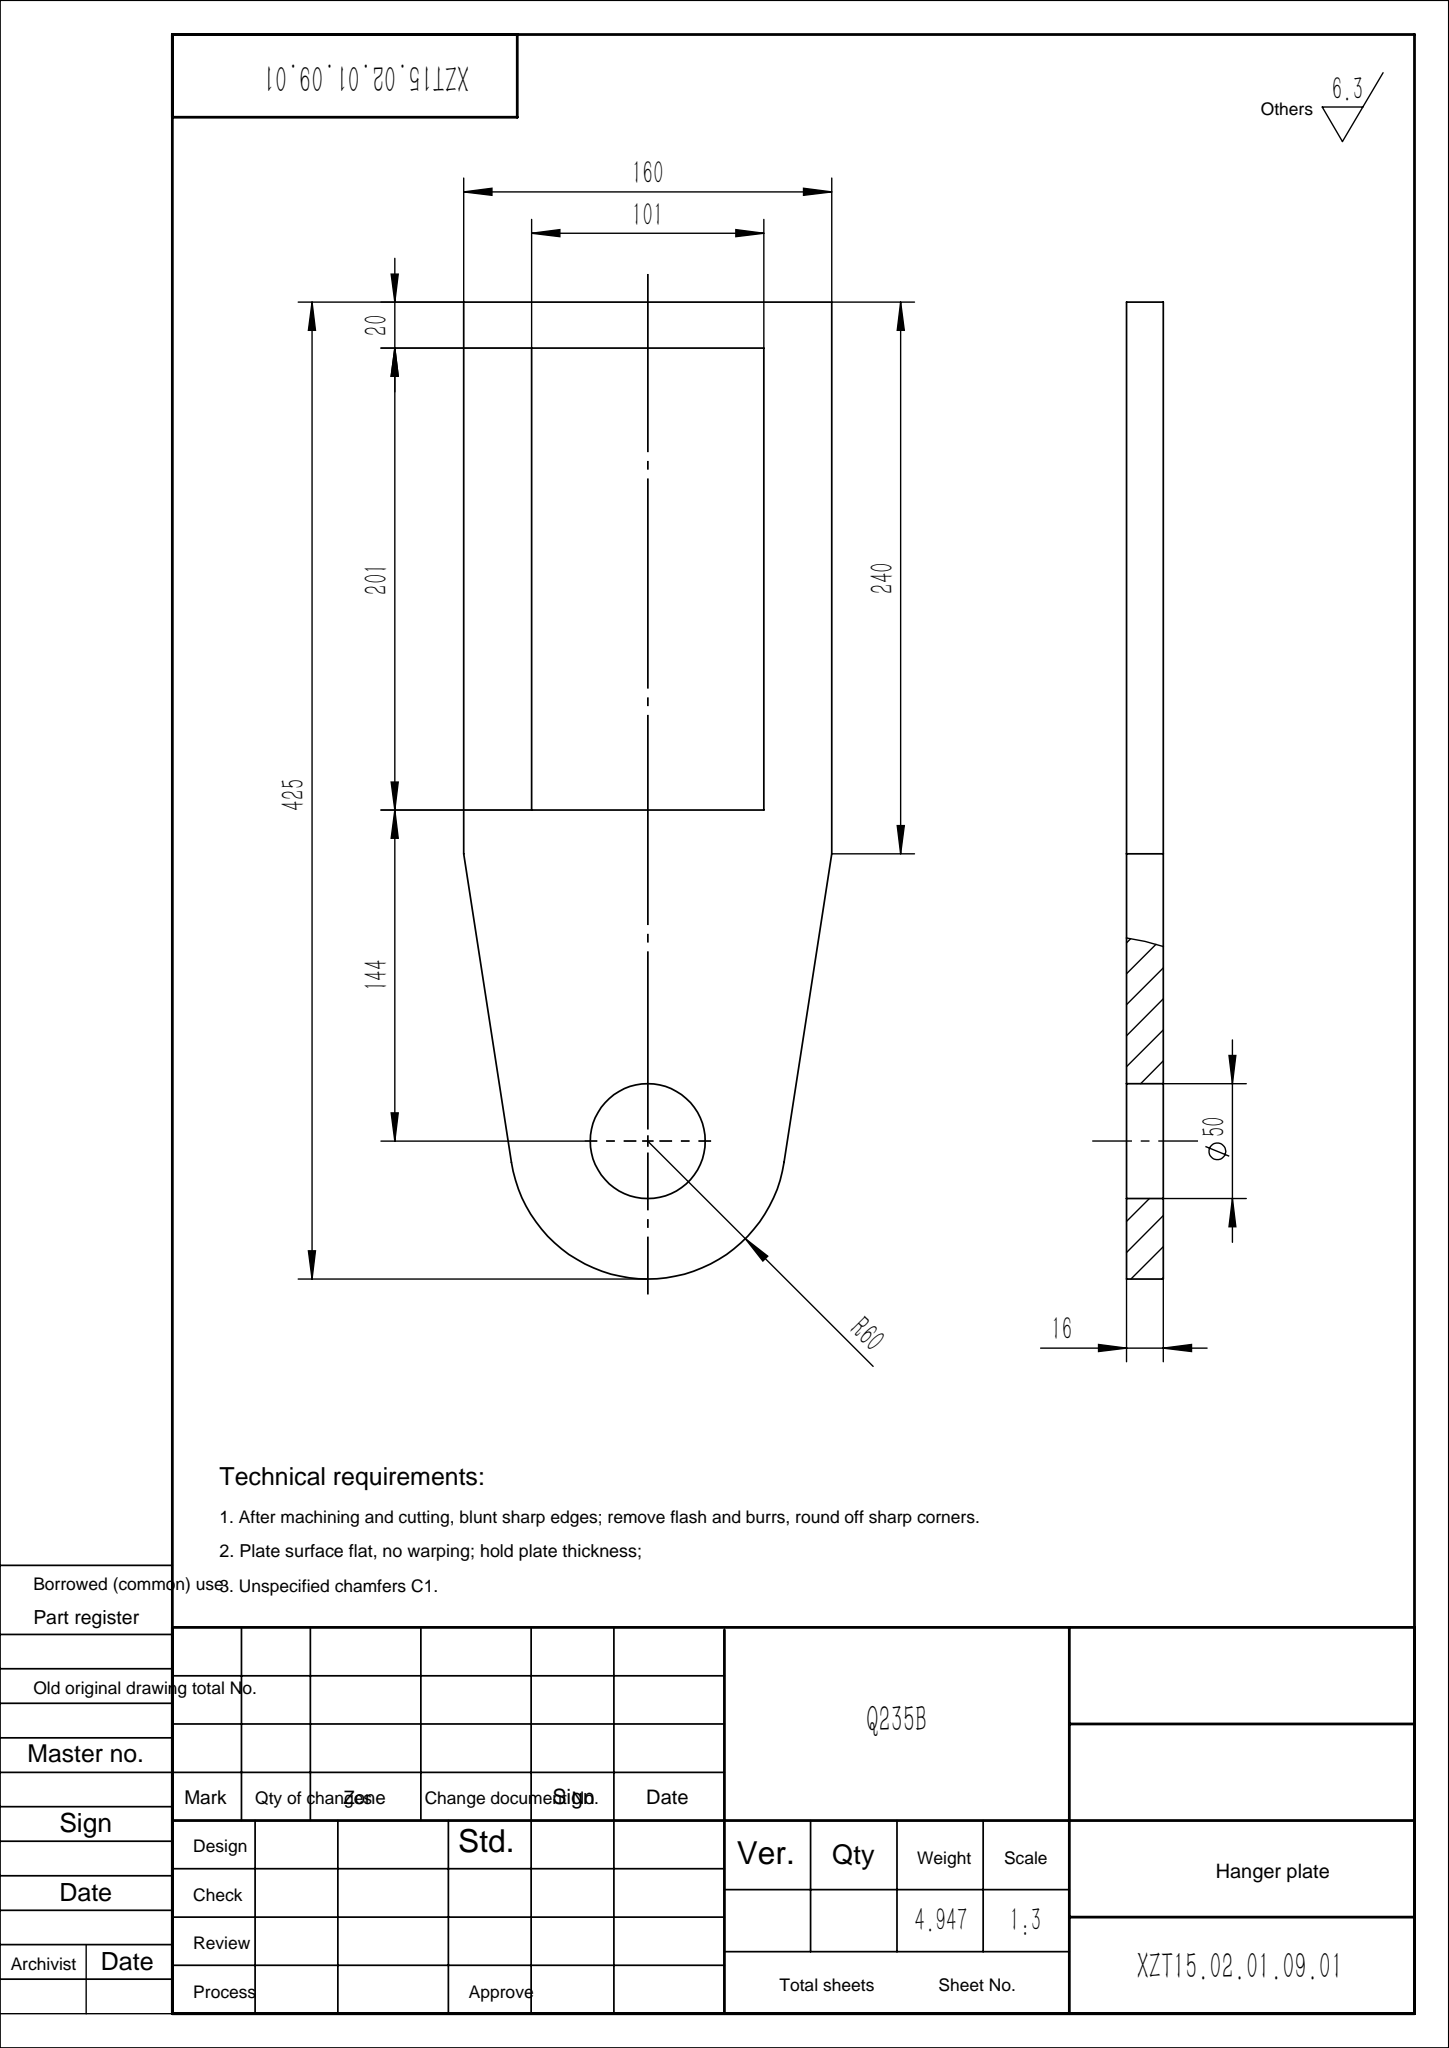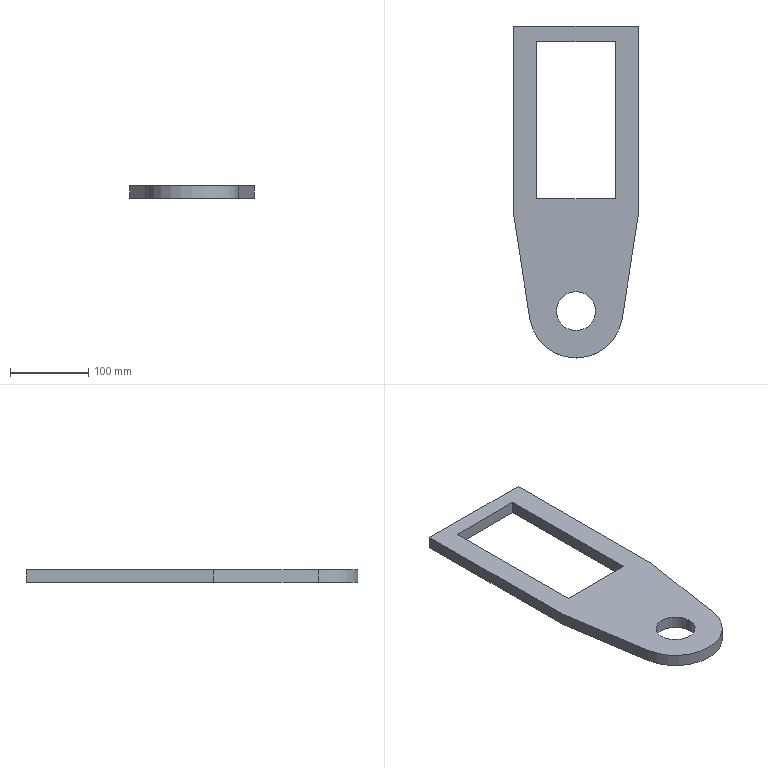Part | SolidWorks | features Extrusion 1 | 1 solid | 14 faces | box 160 x 425 x 16 mm | volume 630136 mm3 | plane 11 | cylinder 3 | commonest cylinder face diameters 50 x2 120 x1
STEP:
#1=CARTESIAN_POINT('',(-25.,0.,8.));
#2=VERTEX_POINT('',#1);
#3=CARTESIAN_POINT('',(25.,0.,8.));
#4=VERTEX_POINT('',#3);
#5=CARTESIAN_POINT('',(0.,0.,8.));
#6=DIRECTION('',(0.,0.,1.));
#7=DIRECTION('',(1.,0.,0.));
#8=AXIS2_PLACEMENT_3D('',#5,#6,#7);
#9=CIRCLE('',#8,25.);
#10=EDGE_CURVE('',#2,#4,#9,.T.);
#11=ORIENTED_EDGE('',*,*,#10,.T.);
#12=CARTESIAN_POINT('',(25.,0.,-8.));
#13=VERTEX_POINT('',#12);
#14=CARTESIAN_POINT('',(25.,0.,8.));
#15=DIRECTION('',(0.,0.,-1.));
#16=VECTOR('',#15,1000.);
#17=LINE('',#14,#16);
#18=EDGE_CURVE('',#4,#13,#17,.T.);
#19=ORIENTED_EDGE('',*,*,#18,.T.);
#20=CARTESIAN_POINT('',(-25.,0.,-8.));
#21=VERTEX_POINT('',#20);
#22=CARTESIAN_POINT('',(0.,0.,-8.));
#23=DIRECTION('',(0.,0.,1.));
#24=DIRECTION('',(1.,0.,0.));
#25=AXIS2_PLACEMENT_3D('',#22,#23,#24);
#26=CIRCLE('',#25,25.);
#27=EDGE_CURVE('',#21,#13,#26,.T.);
#28=ORIENTED_EDGE('',*,*,#27,.F.);
#29=CARTESIAN_POINT('',(-25.,0.,8.));
#30=DIRECTION('',(0.,0.,-1.));
#31=VECTOR('',#30,1000.);
#32=LINE('',#29,#31);
#33=EDGE_CURVE('',#2,#21,#32,.T.);
#34=ORIENTED_EDGE('',*,*,#33,.F.);
#35=EDGE_LOOP('',(#11,#19,#28,#34));
#36=FACE_OUTER_BOUND('',#35,.T.);
#37=CARTESIAN_POINT('',(0.,0.,8.));
#38=DIRECTION('',(0.,0.,-1.));
#39=DIRECTION('',(-1.,0.,0.));
#40=AXIS2_PLACEMENT_3D('',#37,#38,#39);
#41=CYLINDRICAL_SURFACE('',#40,25.);
#42=ADVANCED_FACE('',(#36),#41,.F.);
#43=CARTESIAN_POINT('',(-80.,365.,8.));
#44=VERTEX_POINT('',#43);
#45=CARTESIAN_POINT('',(-80.,125.,8.));
#46=VERTEX_POINT('',#45);
#47=CARTESIAN_POINT('',(-80.,365.,8.));
#48=DIRECTION('',(0.,-1.,0.));
#49=VECTOR('',#48,1000.);
#50=LINE('',#47,#49);
#51=EDGE_CURVE('',#44,#46,#50,.T.);
#52=ORIENTED_EDGE('',*,*,#51,.T.);
#53=CARTESIAN_POINT('',(-59.298,-9.151,8.));
#54=VERTEX_POINT('',#53);
#55=CARTESIAN_POINT('',(-80.,125.,8.));
#56=DIRECTION('',(0.1525,-0.9883,0.));
#57=VECTOR('',#56,1000.);
#58=LINE('',#55,#57);
#59=EDGE_CURVE('',#46,#54,#58,.T.);
#60=ORIENTED_EDGE('',*,*,#59,.T.);
#61=CARTESIAN_POINT('',(59.298,-9.151,8.));
#62=VERTEX_POINT('',#61);
#63=CARTESIAN_POINT('',(0.,0.,8.));
#64=DIRECTION('',(0.,0.,1.));
#65=DIRECTION('',(1.,0.,0.));
#66=AXIS2_PLACEMENT_3D('',#63,#64,#65);
#67=CIRCLE('',#66,60.);
#68=EDGE_CURVE('',#54,#62,#67,.T.);
#69=ORIENTED_EDGE('',*,*,#68,.T.);
#70=CARTESIAN_POINT('',(80.,125.,8.));
#71=VERTEX_POINT('',#70);
#72=CARTESIAN_POINT('',(80.,125.,8.));
#73=DIRECTION('',(0.1525,0.9883,0.));
#74=VECTOR('',#73,1000.);
#75=LINE('',#72,#74);
#76=EDGE_CURVE('',#62,#71,#75,.T.);
#77=ORIENTED_EDGE('',*,*,#76,.T.);
#78=CARTESIAN_POINT('',(80.,365.,8.));
#79=VERTEX_POINT('',#78);
#80=CARTESIAN_POINT('',(80.,365.,8.));
#81=DIRECTION('',(0.,1.,0.));
#82=VECTOR('',#81,1000.);
#83=LINE('',#80,#82);
#84=EDGE_CURVE('',#71,#79,#83,.T.);
#85=ORIENTED_EDGE('',*,*,#84,.T.);
#86=CARTESIAN_POINT('',(80.,365.,8.));
#87=DIRECTION('',(-1.,0.,0.));
#88=VECTOR('',#87,1000.);
#89=LINE('',#86,#88);
#90=EDGE_CURVE('',#79,#44,#89,.T.);
#91=ORIENTED_EDGE('',*,*,#90,.T.);
#92=EDGE_LOOP('',(#52,#60,#69,#77,#85,#91));
#93=FACE_OUTER_BOUND('',#92,.T.);
#94=ORIENTED_EDGE('',*,*,#10,.F.);
#95=CARTESIAN_POINT('',(0.,0.,8.));
#96=DIRECTION('',(0.,0.,1.));
#97=DIRECTION('',(1.,0.,0.));
#98=AXIS2_PLACEMENT_3D('',#95,#96,#97);
#99=CIRCLE('',#98,25.);
#100=EDGE_CURVE('',#4,#2,#99,.T.);
#101=ORIENTED_EDGE('',*,*,#100,.F.);
#102=EDGE_LOOP('',(#94,#101));
#103=FACE_BOUND('',#102,.T.);
#104=CARTESIAN_POINT('',(-50.5,144.,8.));
#105=VERTEX_POINT('',#104);
#106=CARTESIAN_POINT('',(50.5,144.,8.));
#107=VERTEX_POINT('',#106);
#108=CARTESIAN_POINT('',(50.5,144.,8.));
#109=DIRECTION('',(1.,0.,0.));
#110=VECTOR('',#109,1000.);
#111=LINE('',#108,#110);
#112=EDGE_CURVE('',#105,#107,#111,.T.);
#113=ORIENTED_EDGE('',*,*,#112,.F.);
#114=CARTESIAN_POINT('',(-50.5,345.,8.));
#115=VERTEX_POINT('',#114);
#116=CARTESIAN_POINT('',(-50.5,144.,8.));
#117=DIRECTION('',(0.,-1.,0.));
#118=VECTOR('',#117,1000.);
#119=LINE('',#116,#118);
#120=EDGE_CURVE('',#115,#105,#119,.T.);
#121=ORIENTED_EDGE('',*,*,#120,.F.);
#122=CARTESIAN_POINT('',(50.5,345.,8.));
#123=VERTEX_POINT('',#122);
#124=CARTESIAN_POINT('',(50.5,345.,8.));
#125=DIRECTION('',(-1.,0.,0.));
#126=VECTOR('',#125,1000.);
#127=LINE('',#124,#126);
#128=EDGE_CURVE('',#123,#115,#127,.T.);
#129=ORIENTED_EDGE('',*,*,#128,.F.);
#130=CARTESIAN_POINT('',(50.5,144.,8.));
#131=DIRECTION('',(0.,1.,0.));
#132=VECTOR('',#131,1000.);
#133=LINE('',#130,#132);
#134=EDGE_CURVE('',#107,#123,#133,.T.);
#135=ORIENTED_EDGE('',*,*,#134,.F.);
#136=EDGE_LOOP('',(#113,#121,#129,#135));
#137=FACE_BOUND('',#136,.T.);
#138=CARTESIAN_POINT('',(0.,0.,8.));
#139=DIRECTION('',(0.,0.,1.));
#140=DIRECTION('',(1.,0.,0.));
#141=AXIS2_PLACEMENT_3D('',#138,#139,#140);
#142=PLANE('',#141);
#143=ADVANCED_FACE('',(#93,#103,#137),#142,.T.);
#144=ORIENTED_EDGE('',*,*,#27,.T.);
#145=CARTESIAN_POINT('',(0.,0.,-8.));
#146=DIRECTION('',(0.,0.,1.));
#147=DIRECTION('',(1.,0.,0.));
#148=AXIS2_PLACEMENT_3D('',#145,#146,#147);
#149=CIRCLE('',#148,25.);
#150=EDGE_CURVE('',#13,#21,#149,.T.);
#151=ORIENTED_EDGE('',*,*,#150,.T.);
#152=EDGE_LOOP('',(#144,#151));
#153=FACE_BOUND('',#152,.T.);
#154=CARTESIAN_POINT('',(-80.,365.,-8.));
#155=VERTEX_POINT('',#154);
#156=CARTESIAN_POINT('',(-80.,125.,-8.));
#157=VERTEX_POINT('',#156);
#158=CARTESIAN_POINT('',(-80.,365.,-8.));
#159=DIRECTION('',(0.,-1.,0.));
#160=VECTOR('',#159,1000.);
#161=LINE('',#158,#160);
#162=EDGE_CURVE('',#155,#157,#161,.T.);
#163=ORIENTED_EDGE('',*,*,#162,.F.);
#164=CARTESIAN_POINT('',(80.,365.,-8.));
#165=VERTEX_POINT('',#164);
#166=CARTESIAN_POINT('',(80.,365.,-8.));
#167=DIRECTION('',(-1.,0.,0.));
#168=VECTOR('',#167,1000.);
#169=LINE('',#166,#168);
#170=EDGE_CURVE('',#165,#155,#169,.T.);
#171=ORIENTED_EDGE('',*,*,#170,.F.);
#172=CARTESIAN_POINT('',(80.,125.,-8.));
#173=VERTEX_POINT('',#172);
#174=CARTESIAN_POINT('',(80.,365.,-8.));
#175=DIRECTION('',(0.,1.,0.));
#176=VECTOR('',#175,1000.);
#177=LINE('',#174,#176);
#178=EDGE_CURVE('',#173,#165,#177,.T.);
#179=ORIENTED_EDGE('',*,*,#178,.F.);
#180=CARTESIAN_POINT('',(59.298,-9.151,-8.));
#181=VERTEX_POINT('',#180);
#182=CARTESIAN_POINT('',(80.,125.,-8.));
#183=DIRECTION('',(0.1525,0.9883,0.));
#184=VECTOR('',#183,1000.);
#185=LINE('',#182,#184);
#186=EDGE_CURVE('',#181,#173,#185,.T.);
#187=ORIENTED_EDGE('',*,*,#186,.F.);
#188=CARTESIAN_POINT('',(-59.298,-9.151,-8.));
#189=VERTEX_POINT('',#188);
#190=CARTESIAN_POINT('',(0.,0.,-8.));
#191=DIRECTION('',(0.,0.,1.));
#192=DIRECTION('',(-1.,0.,0.));
#193=AXIS2_PLACEMENT_3D('',#190,#191,#192);
#194=CIRCLE('',#193,60.);
#195=EDGE_CURVE('',#189,#181,#194,.T.);
#196=ORIENTED_EDGE('',*,*,#195,.F.);
#197=CARTESIAN_POINT('',(-80.,125.,-8.));
#198=DIRECTION('',(0.1525,-0.9883,0.));
#199=VECTOR('',#198,1000.);
#200=LINE('',#197,#199);
#201=EDGE_CURVE('',#157,#189,#200,.T.);
#202=ORIENTED_EDGE('',*,*,#201,.F.);
#203=EDGE_LOOP('',(#163,#171,#179,#187,#196,#202));
#204=FACE_OUTER_BOUND('',#203,.T.);
#205=CARTESIAN_POINT('',(-50.5,345.,-8.));
#206=VERTEX_POINT('',#205);
#207=CARTESIAN_POINT('',(-50.5,144.,-8.));
#208=VERTEX_POINT('',#207);
#209=CARTESIAN_POINT('',(-50.5,144.,-8.));
#210=DIRECTION('',(0.,-1.,0.));
#211=VECTOR('',#210,1000.);
#212=LINE('',#209,#211);
#213=EDGE_CURVE('',#206,#208,#212,.T.);
#214=ORIENTED_EDGE('',*,*,#213,.T.);
#215=CARTESIAN_POINT('',(50.5,144.,-8.));
#216=VERTEX_POINT('',#215);
#217=CARTESIAN_POINT('',(50.5,144.,-8.));
#218=DIRECTION('',(1.,0.,0.));
#219=VECTOR('',#218,1000.);
#220=LINE('',#217,#219);
#221=EDGE_CURVE('',#208,#216,#220,.T.);
#222=ORIENTED_EDGE('',*,*,#221,.T.);
#223=CARTESIAN_POINT('',(50.5,345.,-8.));
#224=VERTEX_POINT('',#223);
#225=CARTESIAN_POINT('',(50.5,144.,-8.));
#226=DIRECTION('',(0.,1.,0.));
#227=VECTOR('',#226,1000.);
#228=LINE('',#225,#227);
#229=EDGE_CURVE('',#216,#224,#228,.T.);
#230=ORIENTED_EDGE('',*,*,#229,.T.);
#231=CARTESIAN_POINT('',(50.5,345.,-8.));
#232=DIRECTION('',(-1.,0.,0.));
#233=VECTOR('',#232,1000.);
#234=LINE('',#231,#233);
#235=EDGE_CURVE('',#224,#206,#234,.T.);
#236=ORIENTED_EDGE('',*,*,#235,.T.);
#237=EDGE_LOOP('',(#214,#222,#230,#236));
#238=FACE_BOUND('',#237,.T.);
#239=CARTESIAN_POINT('',(0.,0.,-8.));
#240=DIRECTION('',(0.,0.,1.));
#241=DIRECTION('',(1.,0.,0.));
#242=AXIS2_PLACEMENT_3D('',#239,#240,#241);
#243=PLANE('',#242);
#244=ADVANCED_FACE('',(#153,#204,#238),#243,.F.);
#245=ORIENTED_EDGE('',*,*,#162,.T.);
#246=CARTESIAN_POINT('',(-80.,125.,8.));
#247=DIRECTION('',(0.,0.,-1.));
#248=VECTOR('',#247,1000.);
#249=LINE('',#246,#248);
#250=EDGE_CURVE('',#46,#157,#249,.T.);
#251=ORIENTED_EDGE('',*,*,#250,.F.);
#252=ORIENTED_EDGE('',*,*,#51,.F.);
#253=CARTESIAN_POINT('',(-80.,365.,8.));
#254=DIRECTION('',(0.,0.,-1.));
#255=VECTOR('',#254,1000.);
#256=LINE('',#253,#255);
#257=EDGE_CURVE('',#44,#155,#256,.T.);
#258=ORIENTED_EDGE('',*,*,#257,.T.);
#259=EDGE_LOOP('',(#245,#251,#252,#258));
#260=FACE_OUTER_BOUND('',#259,.T.);
#261=CARTESIAN_POINT('',(-80.,365.,8.));
#262=DIRECTION('',(1.,0.,0.));
#263=DIRECTION('',(0.,0.,-1.));
#264=AXIS2_PLACEMENT_3D('',#261,#262,#263);
#265=PLANE('',#264);
#266=ADVANCED_FACE('',(#260),#265,.F.);
#267=ORIENTED_EDGE('',*,*,#201,.T.);
#268=CARTESIAN_POINT('',(-59.298,-9.151,8.));
#269=DIRECTION('',(0.,0.,-1.));
#270=VECTOR('',#269,1000.);
#271=LINE('',#268,#270);
#272=EDGE_CURVE('',#54,#189,#271,.T.);
#273=ORIENTED_EDGE('',*,*,#272,.F.);
#274=ORIENTED_EDGE('',*,*,#59,.F.);
#275=ORIENTED_EDGE('',*,*,#250,.T.);
#276=EDGE_LOOP('',(#267,#273,#274,#275));
#277=FACE_OUTER_BOUND('',#276,.T.);
#278=CARTESIAN_POINT('',(-80.,125.,8.));
#279=DIRECTION('',(0.9883,0.1525,0.));
#280=DIRECTION('',(-0.1525,0.9883,0.));
#281=AXIS2_PLACEMENT_3D('',#278,#279,#280);
#282=PLANE('',#281);
#283=ADVANCED_FACE('',(#277),#282,.F.);
#284=ORIENTED_EDGE('',*,*,#195,.T.);
#285=CARTESIAN_POINT('',(59.298,-9.151,8.));
#286=DIRECTION('',(0.,0.,-1.));
#287=VECTOR('',#286,1000.);
#288=LINE('',#285,#287);
#289=EDGE_CURVE('',#62,#181,#288,.T.);
#290=ORIENTED_EDGE('',*,*,#289,.F.);
#291=ORIENTED_EDGE('',*,*,#68,.F.);
#292=ORIENTED_EDGE('',*,*,#272,.T.);
#293=EDGE_LOOP('',(#284,#290,#291,#292));
#294=FACE_OUTER_BOUND('',#293,.T.);
#295=CARTESIAN_POINT('',(0.,0.,8.));
#296=DIRECTION('',(0.,0.,-1.));
#297=DIRECTION('',(-1.,0.,0.));
#298=AXIS2_PLACEMENT_3D('',#295,#296,#297);
#299=CYLINDRICAL_SURFACE('',#298,60.);
#300=ADVANCED_FACE('',(#294),#299,.T.);
#301=ORIENTED_EDGE('',*,*,#186,.T.);
#302=CARTESIAN_POINT('',(80.,125.,8.));
#303=DIRECTION('',(0.,0.,-1.));
#304=VECTOR('',#303,1000.);
#305=LINE('',#302,#304);
#306=EDGE_CURVE('',#71,#173,#305,.T.);
#307=ORIENTED_EDGE('',*,*,#306,.F.);
#308=ORIENTED_EDGE('',*,*,#76,.F.);
#309=ORIENTED_EDGE('',*,*,#289,.T.);
#310=EDGE_LOOP('',(#301,#307,#308,#309));
#311=FACE_OUTER_BOUND('',#310,.T.);
#312=CARTESIAN_POINT('',(80.,125.,8.));
#313=DIRECTION('',(-0.9883,0.1525,0.));
#314=DIRECTION('',(-0.1525,-0.9883,0.));
#315=AXIS2_PLACEMENT_3D('',#312,#313,#314);
#316=PLANE('',#315);
#317=ADVANCED_FACE('',(#311),#316,.F.);
#318=ORIENTED_EDGE('',*,*,#178,.T.);
#319=CARTESIAN_POINT('',(80.,365.,8.));
#320=DIRECTION('',(0.,0.,-1.));
#321=VECTOR('',#320,1000.);
#322=LINE('',#319,#321);
#323=EDGE_CURVE('',#79,#165,#322,.T.);
#324=ORIENTED_EDGE('',*,*,#323,.F.);
#325=ORIENTED_EDGE('',*,*,#84,.F.);
#326=ORIENTED_EDGE('',*,*,#306,.T.);
#327=EDGE_LOOP('',(#318,#324,#325,#326));
#328=FACE_OUTER_BOUND('',#327,.T.);
#329=CARTESIAN_POINT('',(80.,365.,8.));
#330=DIRECTION('',(-1.,0.,0.));
#331=DIRECTION('',(0.,0.,1.));
#332=AXIS2_PLACEMENT_3D('',#329,#330,#331);
#333=PLANE('',#332);
#334=ADVANCED_FACE('',(#328),#333,.F.);
#335=ORIENTED_EDGE('',*,*,#170,.T.);
#336=ORIENTED_EDGE('',*,*,#257,.F.);
#337=ORIENTED_EDGE('',*,*,#90,.F.);
#338=ORIENTED_EDGE('',*,*,#323,.T.);
#339=EDGE_LOOP('',(#335,#336,#337,#338));
#340=FACE_OUTER_BOUND('',#339,.T.);
#341=CARTESIAN_POINT('',(80.,365.,8.));
#342=DIRECTION('',(0.,-1.,0.));
#343=DIRECTION('',(0.,0.,-1.));
#344=AXIS2_PLACEMENT_3D('',#341,#342,#343);
#345=PLANE('',#344);
#346=ADVANCED_FACE('',(#340),#345,.F.);
#347=ORIENTED_EDGE('',*,*,#18,.F.);
#348=ORIENTED_EDGE('',*,*,#100,.T.);
#349=ORIENTED_EDGE('',*,*,#33,.T.);
#350=ORIENTED_EDGE('',*,*,#150,.F.);
#351=EDGE_LOOP('',(#347,#348,#349,#350));
#352=FACE_OUTER_BOUND('',#351,.T.);
#353=CARTESIAN_POINT('',(0.,0.,8.));
#354=DIRECTION('',(0.,0.,-1.));
#355=DIRECTION('',(-1.,0.,0.));
#356=AXIS2_PLACEMENT_3D('',#353,#354,#355);
#357=CYLINDRICAL_SURFACE('',#356,25.);
#358=ADVANCED_FACE('',(#352),#357,.F.);
#359=ORIENTED_EDGE('',*,*,#213,.F.);
#360=CARTESIAN_POINT('',(-50.5,345.,8.));
#361=DIRECTION('',(0.,0.,-1.));
#362=VECTOR('',#361,1000.);
#363=LINE('',#360,#362);
#364=EDGE_CURVE('',#115,#206,#363,.T.);
#365=ORIENTED_EDGE('',*,*,#364,.F.);
#366=ORIENTED_EDGE('',*,*,#120,.T.);
#367=CARTESIAN_POINT('',(-50.5,144.,8.));
#368=DIRECTION('',(0.,0.,-1.));
#369=VECTOR('',#368,1000.);
#370=LINE('',#367,#369);
#371=EDGE_CURVE('',#105,#208,#370,.T.);
#372=ORIENTED_EDGE('',*,*,#371,.T.);
#373=EDGE_LOOP('',(#359,#365,#366,#372));
#374=FACE_OUTER_BOUND('',#373,.T.);
#375=CARTESIAN_POINT('',(-50.5,144.,8.));
#376=DIRECTION('',(1.,0.,0.));
#377=DIRECTION('',(0.,0.,-1.));
#378=AXIS2_PLACEMENT_3D('',#375,#376,#377);
#379=PLANE('',#378);
#380=ADVANCED_FACE('',(#374),#379,.T.);
#381=ORIENTED_EDGE('',*,*,#221,.F.);
#382=ORIENTED_EDGE('',*,*,#371,.F.);
#383=ORIENTED_EDGE('',*,*,#112,.T.);
#384=CARTESIAN_POINT('',(50.5,144.,8.));
#385=DIRECTION('',(0.,0.,-1.));
#386=VECTOR('',#385,1000.);
#387=LINE('',#384,#386);
#388=EDGE_CURVE('',#107,#216,#387,.T.);
#389=ORIENTED_EDGE('',*,*,#388,.T.);
#390=EDGE_LOOP('',(#381,#382,#383,#389));
#391=FACE_OUTER_BOUND('',#390,.T.);
#392=CARTESIAN_POINT('',(50.5,144.,8.));
#393=DIRECTION('',(0.,1.,0.));
#394=DIRECTION('',(0.,0.,1.));
#395=AXIS2_PLACEMENT_3D('',#392,#393,#394);
#396=PLANE('',#395);
#397=ADVANCED_FACE('',(#391),#396,.T.);
#398=ORIENTED_EDGE('',*,*,#229,.F.);
#399=ORIENTED_EDGE('',*,*,#388,.F.);
#400=ORIENTED_EDGE('',*,*,#134,.T.);
#401=CARTESIAN_POINT('',(50.5,345.,8.));
#402=DIRECTION('',(0.,0.,-1.));
#403=VECTOR('',#402,1000.);
#404=LINE('',#401,#403);
#405=EDGE_CURVE('',#123,#224,#404,.T.);
#406=ORIENTED_EDGE('',*,*,#405,.T.);
#407=EDGE_LOOP('',(#398,#399,#400,#406));
#408=FACE_OUTER_BOUND('',#407,.T.);
#409=CARTESIAN_POINT('',(50.5,144.,8.));
#410=DIRECTION('',(-1.,0.,0.));
#411=DIRECTION('',(0.,0.,1.));
#412=AXIS2_PLACEMENT_3D('',#409,#410,#411);
#413=PLANE('',#412);
#414=ADVANCED_FACE('',(#408),#413,.T.);
#415=ORIENTED_EDGE('',*,*,#235,.F.);
#416=ORIENTED_EDGE('',*,*,#405,.F.);
#417=ORIENTED_EDGE('',*,*,#128,.T.);
#418=ORIENTED_EDGE('',*,*,#364,.T.);
#419=EDGE_LOOP('',(#415,#416,#417,#418));
#420=FACE_OUTER_BOUND('',#419,.T.);
#421=CARTESIAN_POINT('',(50.5,345.,8.));
#422=DIRECTION('',(0.,-1.,0.));
#423=DIRECTION('',(0.,0.,-1.));
#424=AXIS2_PLACEMENT_3D('',#421,#422,#423);
#425=PLANE('',#424);
#426=ADVANCED_FACE('',(#420),#425,.T.);
#427=CLOSED_SHELL('',(#42,#143,#244,#266,#283,#300,#317,#334,#346,#358,#380,#397,#414,#426));
#428=MANIFOLD_SOLID_BREP('',#427);
#429=CARTESIAN_POINT('',(0.,0.,0.));
#430=DIRECTION('',(0.,0.,1.));
#431=DIRECTION('',(1.,0.,0.));
#432=AXIS2_PLACEMENT_3D('',#429,#430,#431);
#433=(LENGTH_UNIT()NAMED_UNIT(*)SI_UNIT(.MILLI.,.METRE.));
#434=UNCERTAINTY_MEASURE_WITH_UNIT(LENGTH_MEASURE(0.00001),#433,'','');
#435=(NAMED_UNIT(*)PLANE_ANGLE_UNIT()SI_UNIT($,.RADIAN.));
#436=(NAMED_UNIT(*)SI_UNIT($,.STERADIAN.)SOLID_ANGLE_UNIT());
#437=(GEOMETRIC_REPRESENTATION_CONTEXT(3)GLOBAL_UNCERTAINTY_ASSIGNED_CONTEXT((#434))GLOBAL_UNIT_ASSIGNED_CONTEXT((#433,#435,#436))REPRESENTATION_CONTEXT('',''));
#438=ADVANCED_BREP_SHAPE_REPRESENTATION('',(#428,#432),#437);